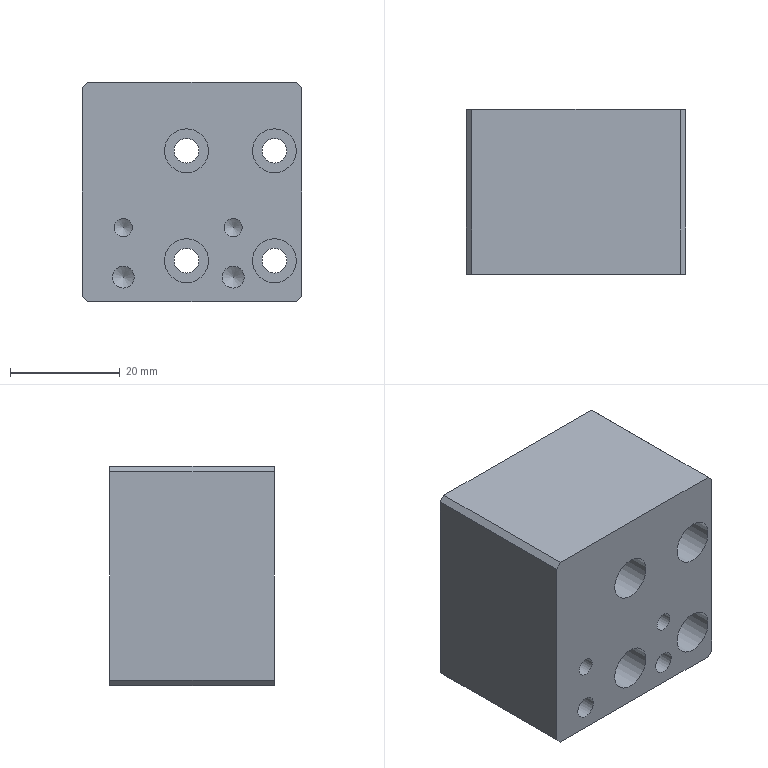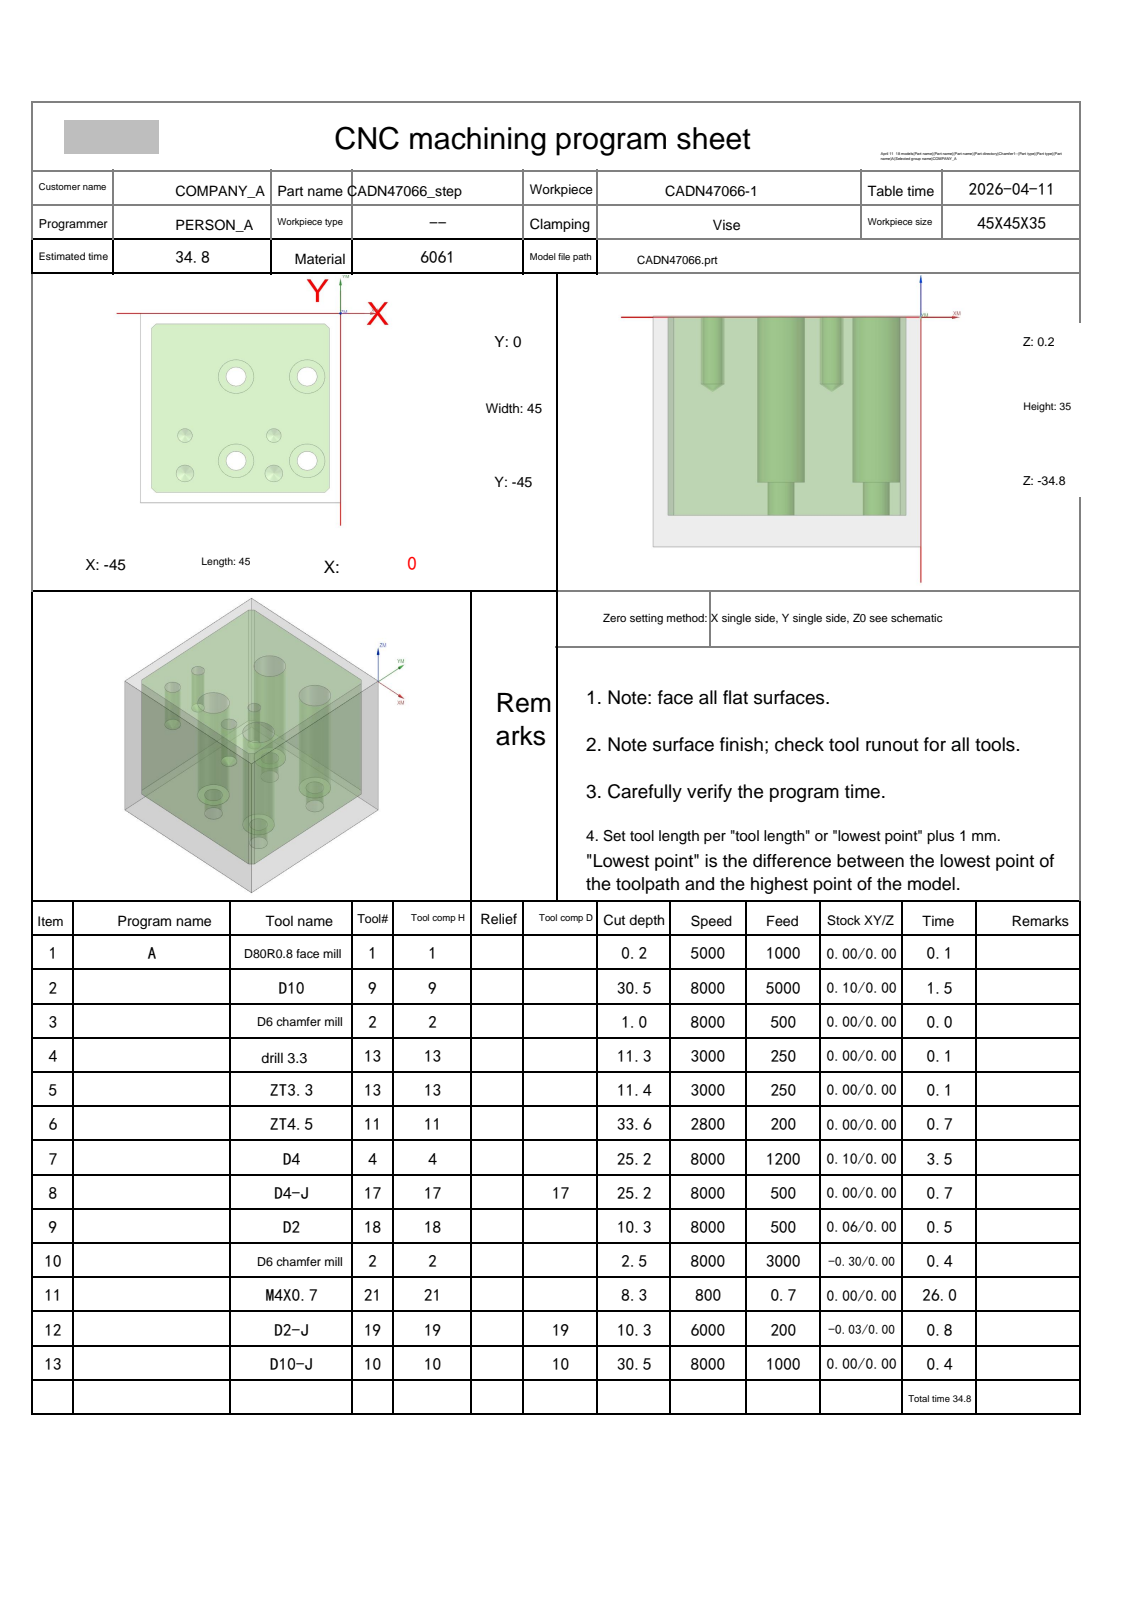NC program | NX | posted by the shop | part box 40 x 30 x 40 mm
Whole program, first 1145 of 1681 lines:
%
O0001
(Machine time: 60.64 MIN)
(===Total Tool:11===)
(T1=D80R0.8 face mill D=80.  R=0.8  D-  H01 Z=0.    )
(T9=D10     D=10.  R=0.   D-  H09 Z=-30.3 )
(T2=D6 chamfer mill   D=6.   R=0.   D-  H02 Z=-2.3  )
(T13=drill 3.3  D=3.3  DR_a=118 D-  H13 Z=-11.2 )
(T11=ZT4.5  D=4.5  DR_a=118 D-  H11 Z=-33.35)
(T4=D4      D=4.   R=0.   D-  H04 Z=-25.  )
(T17=D4-J   D=4.   R=0.   D17 H17 Z=-25.  )
(T18=D2     D=2.   R=0.   D-  H18 Z=-10.1 )
(T21=M4X0.7 D=3.3  DR_a=180 D-  H21 Z=-8.1  )
(T19=D2-J   D=2.   R=0.   D19 H19 Z=-10.1 )
(T10=D10-J  D=10.  R=0.   D10 H10 Z=-30.3 )
G80 G90 G17 G49 G40
G91 G28 Z0
M01
N1 T01 M06
(D80R0.8 face mill  D=80. R=0.8 H=01 ce=0.00 di=0.00)
G00 G90 G54 X42.5 Y-22.5 M03 S5000
G43 H01 Z20.
M08
Z2.
G01 Z0.0 F1000.
X37.5
X-82.5
X-87.5
Z2.
G00 Z20.
G91 G28 Z0.0
M05
M09
G91 G28 Z0.0
M01
N2 T09 M06
(D10  D=10. R=0. H=09 ce=0.10 di=0.00)
G00 G90 G54 X2.6 Y-22.5 M03 S8000
G43 H09 Z20.
M08
Z.5
G01 Y-41.5 Z.421 F5000.
G02 X1.106 Y-45.106 Z.404 I-5.1 J0.0
G01 X.106 Y-46.106 Z.398
G02 X-3.5 Y-47.6 Z.382 I-3.606 J3.606
G01 X-41.5 Z.223
G02 X-45.106 Y-46.106 Z.207 I0.0 J5.1
G01 X-46.106 Y-45.106 Z.201
G02 X-47.6 Y-41.5 Z.184 I3.606 J3.606
G01 Y-3.5 Z.026
G02 X-46.106 Y.106 Z.009 I5.1 J0.0
G01 X-45.106 Y1.106 Z.003
G02 X-41.5 Y2.6 Z-.013 I3.606 J-3.606
G01 X-3.5 Z-.171
G02 X.106 Y1.106 Z-.188 I0.0 J-5.1
G01 X1.106 Y.106 Z-.194
G02 X2.6 Y-3.5 Z-.211 I-3.606 J-3.606
G01 Y-41.5 Z-.369
G02 X1.106 Y-45.106 Z-.386 I-5.1 J0.0
G01 X.106 Y-46.106 Z-.391
G02 X-3.5 Y-47.6 Z-.408 I-3.606 J3.606
G01 X-41.5 Z-.566
G02 X-45.106 Y-46.106 Z-.583 I0.0 J5.1
G01 X-46.106 Y-45.106 Z-.589
G02 X-47.6 Y-41.5 Z-.606 I3.606 J3.606
G01 Y-3.5 Z-.764
G02 X-46.106 Y.106 Z-.78 I5.1 J0.0
G01 X-45.106 Y1.106 Z-.786
G02 X-41.5 Y2.6 Z-.803 I3.606 J-3.606
G01 X-3.5 Z-.961
G02 X.106 Y1.106 Z-.978 I0.0 J-5.1
G01 X1.106 Y.106 Z-.984
G02 X2.6 Y-3.5 Z-1. I-3.606 J-3.606
G01 Y-41.5 Z-1.159
G02 X1.106 Y-45.106 Z-1.175 I-5.1 J0.0
G01 X.106 Y-46.106 Z-1.181
G02 X-3.5 Y-47.6 Z-1.198 I-3.606 J3.606
G01 X-41.5 Z-1.356
G02 X-45.106 Y-46.106 Z-1.373 I0.0 J5.1
G01 X-46.106 Y-45.106 Z-1.379
G02 X-47.6 Y-41.5 Z-1.395 I3.606 J3.606
G01 Y-3.5 Z-1.553
G02 X-46.106 Y.106 Z-1.57 I5.1 J0.0
G01 X-45.106 Y1.106 Z-1.576
G02 X-41.5 Y2.6 Z-1.593 I3.606 J-3.606
G01 X-3.5 Z-1.751
G02 X.106 Y1.106 Z-1.768 I0.0 J-5.1
G01 X1.106 Y.106 Z-1.773
G02 X2.6 Y-3.5 Z-1.79 I-3.606 J-3.606
G01 Y-41.5 Z-1.948
G02 X1.106 Y-45.106 Z-1.965 I-5.1 J0.0
G01 X.106 Y-46.106 Z-1.971
G02 X-3.5 Y-47.6 Z-1.988 I-3.606 J3.606
G01 X-41.5 Z-2.146
G02 X-45.106 Y-46.106 Z-2.162 I0.0 J5.1
G01 X-46.106 Y-45.106 Z-2.168
G02 X-47.6 Y-41.5 Z-2.185 I3.606 J3.606
G01 Y-3.5 Z-2.343
G02 X-46.106 Y.106 Z-2.36 I5.1 J0.0
G01 X-45.106 Y1.106 Z-2.366
G02 X-41.5 Y2.6 Z-2.382 I3.606 J-3.606
G01 X-3.5 Z-2.541
G02 X.106 Y1.106 Z-2.557 I0.0 J-5.1
G01 X1.106 Y.106 Z-2.563
G02 X2.6 Y-3.5 Z-2.58 I-3.606 J-3.606
G01 Y-41.5 Z-2.738
G02 X1.106 Y-45.106 Z-2.755 I-5.1 J0.0
G01 X.106 Y-46.106 Z-2.761
G02 X-3.5 Y-47.6 Z-2.777 I-3.606 J3.606
G01 X-41.5 Z-2.936
G02 X-45.106 Y-46.106 Z-2.952 I0.0 J5.1
G01 X-46.106 Y-45.106 Z-2.958
G02 X-47.6 Y-41.5 Z-2.975 I3.606 J3.606
G01 Y-3.5 Z-3.133
G02 X-46.106 Y.106 Z-3.15 I5.1 J0.0
G01 X-45.106 Y1.106 Z-3.156
G02 X-41.5 Y2.6 Z-3.172 I3.606 J-3.606
G01 X-3.5 Z-3.33
G02 X.106 Y1.106 Z-3.347 I0.0 J-5.1
G01 X1.106 Y.106 Z-3.353
G02 X2.6 Y-3.5 Z-3.37 I-3.606 J-3.606
G01 Y-41.5 Z-3.528
G02 X1.106 Y-45.106 Z-3.544 I-5.1 J0.0
G01 X.106 Y-46.106 Z-3.55
G02 X-3.5 Y-47.6 Z-3.567 I-3.606 J3.606
G01 X-41.5 Z-3.725
G02 X-45.106 Y-46.106 Z-3.742 I0.0 J5.1
G01 X-46.106 Y-45.106 Z-3.748
G02 X-47.6 Y-41.5 Z-3.764 I3.606 J3.606
G01 Y-3.5 Z-3.923
G02 X-46.106 Y.106 Z-3.939 I5.1 J0.0
G01 X-45.106 Y1.106 Z-3.945
G02 X-41.5 Y2.6 Z-3.962 I3.606 J-3.606
G01 X-3.5 Z-4.12
G02 X.106 Y1.106 Z-4.137 I0.0 J-5.1
G01 X1.106 Y.106 Z-4.143
G02 X2.6 Y-3.5 Z-4.159 I-3.606 J-3.606
G01 Y-41.5 Z-4.318
G02 X1.106 Y-45.106 Z-4.334 I-5.1 J0.0
G01 X.106 Y-46.106 Z-4.34
G02 X-3.5 Y-47.6 Z-4.357 I-3.606 J3.606
G01 X-41.5 Z-4.515
G02 X-45.106 Y-46.106 Z-4.532 I0.0 J5.1
G01 X-46.106 Y-45.106 Z-4.538
G02 X-47.6 Y-41.5 Z-4.554 I3.606 J3.606
G01 Y-3.5 Z-4.712
G02 X-46.106 Y.106 Z-4.729 I5.1 J0.0
G01 X-45.106 Y1.106 Z-4.735
G02 X-41.5 Y2.6 Z-4.752 I3.606 J-3.606
G01 X-3.5 Z-4.91
G02 X.106 Y1.106 Z-4.927 I0.0 J-5.1
G01 X1.106 Y.106 Z-4.932
G02 X2.6 Y-3.5 Z-4.949 I-3.606 J-3.606
G01 Y-41.5 Z-5.107
G02 X1.106 Y-45.106 Z-5.124 I-5.1 J0.0
G01 X.106 Y-46.106 Z-5.13
G02 X-3.5 Y-47.6 Z-5.147 I-3.606 J3.606
G01 X-41.5 Z-5.305
G02 X-45.106 Y-46.106 Z-5.321 I0.0 J5.1
G01 X-46.106 Y-45.106 Z-5.327
G02 X-47.6 Y-41.5 Z-5.344 I3.606 J3.606
G01 Y-3.5 Z-5.502
G02 X-46.106 Y.106 Z-5.519 I5.1 J0.0
G01 X-45.106 Y1.106 Z-5.525
G02 X-41.5 Y2.6 Z-5.541 I3.606 J-3.606
G01 X-3.5 Z-5.7
G02 X.106 Y1.106 Z-5.716 I0.0 J-5.1
G01 X1.106 Y.106 Z-5.722
G02 X2.6 Y-3.5 Z-5.739 I-3.606 J-3.606
G01 Y-41.5 Z-5.897
G02 X1.106 Y-45.106 Z-5.914 I-5.1 J0.0
G01 X.106 Y-46.106 Z-5.92
G02 X-3.5 Y-47.6 Z-5.936 I-3.606 J3.606
G01 X-41.5 Z-6.094
G02 X-45.106 Y-46.106 Z-6.111 I0.0 J5.1
G01 X-46.106 Y-45.106 Z-6.117
G02 X-47.6 Y-41.5 Z-6.134 I3.606 J3.606
G01 Y-3.5 Z-6.292
G02 X-46.106 Y.106 Z-6.309 I5.1 J0.0
G01 X-45.106 Y1.106 Z-6.314
G02 X-41.5 Y2.6 Z-6.331 I3.606 J-3.606
G01 X-3.5 Z-6.489
G02 X.106 Y1.106 Z-6.506 I0.0 J-5.1
G01 X1.106 Y.106 Z-6.512
G02 X2.6 Y-3.5 Z-6.529 I-3.606 J-3.606
G01 Y-41.5 Z-6.687
G02 X1.106 Y-45.106 Z-6.703 I-5.1 J0.0
G01 X.106 Y-46.106 Z-6.709
G02 X-3.5 Y-47.6 Z-6.726 I-3.606 J3.606
G01 X-41.5 Z-6.884
G02 X-45.106 Y-46.106 Z-6.901 I0.0 J5.1
G01 X-46.106 Y-45.106 Z-6.907
G02 X-47.6 Y-41.5 Z-6.923 I3.606 J3.606
G01 Y-3.5 Z-7.082
G02 X-46.106 Y.106 Z-7.098 I5.1 J0.0
G01 X-45.106 Y1.106 Z-7.104
G02 X-41.5 Y2.6 Z-7.121 I3.606 J-3.606
G01 X-3.5 Z-7.279
G02 X.106 Y1.106 Z-7.296 I0.0 J-5.1
G01 X1.106 Y.106 Z-7.302
G02 X2.6 Y-3.5 Z-7.318 I-3.606 J-3.606
G01 Y-41.5 Z-7.477
G02 X1.106 Y-45.106 Z-7.493 I-5.1 J0.0
G01 X.106 Y-46.106 Z-7.499
G02 X-3.5 Y-47.6 Z-7.516 I-3.606 J3.606
G01 X-41.5 Z-7.674
G02 X-45.106 Y-46.106 Z-7.691 I0.0 J5.1
G01 X-46.106 Y-45.106 Z-7.697
G02 X-47.6 Y-41.5 Z-7.713 I3.606 J3.606
G01 Y-3.5 Z-7.871
G02 X-46.106 Y.106 Z-7.888 I5.1 J0.0
G01 X-45.106 Y1.106 Z-7.894
G02 X-41.5 Y2.6 Z-7.911 I3.606 J-3.606
G01 X-3.5 Z-8.069
G02 X.106 Y1.106 Z-8.086 I0.0 J-5.1
G01 X1.106 Y.106 Z-8.091
G02 X2.6 Y-3.5 Z-8.108 I-3.606 J-3.606
G01 Y-41.5 Z-8.266
G02 X1.106 Y-45.106 Z-8.283 I-5.1 J0.0
G01 X.106 Y-46.106 Z-8.289
G02 X-3.5 Y-47.6 Z-8.306 I-3.606 J3.606
G01 X-41.5 Z-8.464
G02 X-45.106 Y-46.106 Z-8.48 I0.0 J5.1
G01 X-46.106 Y-45.106 Z-8.486
G02 X-47.6 Y-41.5 Z-8.503 I3.606 J3.606
G01 Y-3.5 Z-8.661
G02 X-46.106 Y.106 Z-8.678 I5.1 J0.0
G01 X-45.106 Y1.106 Z-8.684
G02 X-41.5 Y2.6 Z-8.7 I3.606 J-3.606
G01 X-3.5 Z-8.859
G02 X.106 Y1.106 Z-8.875 I0.0 J-5.1
G01 X1.106 Y.106 Z-8.881
G02 X2.6 Y-3.5 Z-8.898 I-3.606 J-3.606
G01 Y-41.5 Z-9.056
G02 X1.106 Y-45.106 Z-9.073 I-5.1 J0.0
G01 X.106 Y-46.106 Z-9.079
G02 X-3.5 Y-47.6 Z-9.095 I-3.606 J3.606
G01 X-41.5 Z-9.253
G02 X-45.106 Y-46.106 Z-9.27 I0.0 J5.1
G01 X-46.106 Y-45.106 Z-9.276
G02 X-47.6 Y-41.5 Z-9.293 I3.606 J3.606
G01 Y-3.5 Z-9.451
G02 X-46.106 Y.106 Z-9.468 I5.1 J0.0
G01 X-45.106 Y1.106 Z-9.473
G02 X-41.5 Y2.6 Z-9.49 I3.606 J-3.606
G01 X-3.5 Z-9.648
G02 X.106 Y1.106 Z-9.665 I0.0 J-5.1
G01 X1.106 Y.106 Z-9.671
G02 X2.6 Y-3.5 Z-9.688 I-3.606 J-3.606
G01 Y-41.5 Z-9.846
G02 X1.106 Y-45.106 Z-9.862 I-5.1 J0.0
G01 X.106 Y-46.106 Z-9.868
G02 X-3.5 Y-47.6 Z-9.885 I-3.606 J3.606
G01 X-41.5 Z-10.043
G02 X-45.106 Y-46.106 Z-10.06 I0.0 J5.1
G01 X-46.106 Y-45.106 Z-10.066
G02 X-47.6 Y-41.5 Z-10.082 I3.606 J3.606
G01 Y-3.5 Z-10.241
G02 X-46.106 Y.106 Z-10.257 I5.1 J0.0
G01 X-45.106 Y1.106 Z-10.263
G02 X-41.5 Y2.6 Z-10.28 I3.606 J-3.606
G01 X-3.5 Z-10.438
G02 X.106 Y1.106 Z-10.455 I0.0 J-5.1
G01 X1.106 Y.106 Z-10.461
G02 X2.6 Y-3.5 Z-10.477 I-3.606 J-3.606
G01 Y-41.5 Z-10.636
G02 X1.106 Y-45.106 Z-10.652 I-5.1 J0.0
G01 X.106 Y-46.106 Z-10.658
G02 X-3.5 Y-47.6 Z-10.675 I-3.606 J3.606
G01 X-41.5 Z-10.833
G02 X-45.106 Y-46.106 Z-10.85 I0.0 J5.1
G01 X-46.106 Y-45.106 Z-10.856
G02 X-47.6 Y-41.5 Z-10.872 I3.606 J3.606
G01 Y-3.5 Z-11.03
G02 X-46.106 Y.106 Z-11.047 I5.1 J0.0
G01 X-45.106 Y1.106 Z-11.053
G02 X-41.5 Y2.6 Z-11.07 I3.606 J-3.606
G01 X-3.5 Z-11.228
G02 X.106 Y1.106 Z-11.244 I0.0 J-5.1
G01 X1.106 Y.106 Z-11.25
G02 X2.6 Y-3.5 Z-11.267 I-3.606 J-3.606
G01 Y-41.5 Z-11.425
G02 X1.106 Y-45.106 Z-11.442 I-5.1 J0.0
G01 X.106 Y-46.106 Z-11.448
G02 X-3.5 Y-47.6 Z-11.464 I-3.606 J3.606
G01 X-41.5 Z-11.623
G02 X-45.106 Y-46.106 Z-11.639 I0.0 J5.1
G01 X-46.106 Y-45.106 Z-11.645
G02 X-47.6 Y-41.5 Z-11.662 I3.606 J3.606
G01 Y-3.5 Z-11.82
G02 X-46.106 Y.106 Z-11.837 I5.1 J0.0
G01 X-45.106 Y1.106 Z-11.843
G02 X-41.5 Y2.6 Z-11.859 I3.606 J-3.606
G01 X-3.5 Z-12.018
G02 X.106 Y1.106 Z-12.034 I0.0 J-5.1
G01 X1.106 Y.106 Z-12.04
G02 X2.6 Y-3.5 Z-12.057 I-3.606 J-3.606
G01 Y-41.5 Z-12.215
G02 X1.106 Y-45.106 Z-12.232 I-5.1 J0.0
G01 X.106 Y-46.106 Z-12.238
G02 X-3.5 Y-47.6 Z-12.254 I-3.606 J3.606
G01 X-41.5 Z-12.412
G02 X-45.106 Y-46.106 Z-12.429 I0.0 J5.1
G01 X-46.106 Y-45.106 Z-12.435
G02 X-47.6 Y-41.5 Z-12.452 I3.606 J3.606
G01 Y-3.5 Z-12.61
G02 X-46.106 Y.106 Z-12.627 I5.1 J0.0
G01 X-45.106 Y1.106 Z-12.632
G02 X-41.5 Y2.6 Z-12.649 I3.606 J-3.606
G01 X-3.5 Z-12.807
G02 X.106 Y1.106 Z-12.824 I0.0 J-5.1
G01 X1.106 Y.106 Z-12.83
G02 X2.6 Y-3.5 Z-12.847 I-3.606 J-3.606
G01 Y-41.5 Z-13.005
G02 X1.106 Y-45.106 Z-13.021 I-5.1 J0.0
G01 X.106 Y-46.106 Z-13.027
G02 X-3.5 Y-47.6 Z-13.044 I-3.606 J3.606
G01 X-41.5 Z-13.202
G02 X-45.106 Y-46.106 Z-13.219 I0.0 J5.1
G01 X-46.106 Y-45.106 Z-13.225
G02 X-47.6 Y-41.5 Z-13.241 I3.606 J3.606
G01 Y-3.5 Z-13.4
G02 X-46.106 Y.106 Z-13.416 I5.1 J0.0
G01 X-45.106 Y1.106 Z-13.422
G02 X-41.5 Y2.6 Z-13.439 I3.606 J-3.606
G01 X-3.5 Z-13.597
G02 X.106 Y1.106 Z-13.614 I0.0 J-5.1
G01 X1.106 Y.106 Z-13.62
G02 X2.6 Y-3.5 Z-13.636 I-3.606 J-3.606
G01 Y-41.5 Z-13.794
G02 X1.106 Y-45.106 Z-13.811 I-5.1 J0.0
G01 X.106 Y-46.106 Z-13.817
G02 X-3.5 Y-47.6 Z-13.834 I-3.606 J3.606
G01 X-41.5 Z-13.992
G02 X-45.106 Y-46.106 Z-14.009 I0.0 J5.1
G01 X-46.106 Y-45.106 Z-14.014
G02 X-47.6 Y-41.5 Z-14.031 I3.606 J3.606
G01 Y-3.5 Z-14.189
G02 X-46.106 Y.106 Z-14.206 I5.1 J0.0
G01 X-45.106 Y1.106 Z-14.212
G02 X-41.5 Y2.6 Z-14.229 I3.606 J-3.606
G01 X-3.5 Z-14.387
G02 X.106 Y1.106 Z-14.403 I0.0 J-5.1
G01 X1.106 Y.106 Z-14.409
G02 X2.6 Y-3.5 Z-14.426 I-3.606 J-3.606
G01 Y-41.5 Z-14.584
G02 X1.106 Y-45.106 Z-14.601 I-5.1 J0.0
G01 X.106 Y-46.106 Z-14.607
G02 X-3.5 Y-47.6 Z-14.623 I-3.606 J3.606
G01 X-41.5 Z-14.782
G02 X-45.106 Y-46.106 Z-14.798 I0.0 J5.1
G01 X-46.106 Y-45.106 Z-14.804
G02 X-47.6 Y-41.5 Z-14.821 I3.606 J3.606
G01 Y-3.5 Z-14.979
G02 X-46.106 Y.106 Z-14.996 I5.1 J0.0
G01 X-45.106 Y1.106 Z-15.002
G02 X-41.5 Y2.6 Z-15.018 I3.606 J-3.606
G01 X-3.5 Z-15.177
G02 X.106 Y1.106 Z-15.193 I0.0 J-5.1
G01 X1.106 Y.106 Z-15.199
G02 X2.6 Y-3.5 Z-15.216 I-3.606 J-3.606
G01 Y-41.5 Z-15.374
G02 X1.106 Y-45.106 Z-15.391 I-5.1 J0.0
G01 X.106 Y-46.106 Z-15.397
G02 X-3.5 Y-47.6 Z-15.413 I-3.606 J3.606
G01 X-41.5 Z-15.571
G02 X-45.106 Y-46.106 Z-15.588 I0.0 J5.1
G01 X-46.106 Y-45.106 Z-15.594
G02 X-47.6 Y-41.5 Z-15.611 I3.606 J3.606
G01 Y-3.5 Z-15.769
G02 X-46.106 Y.106 Z-15.786 I5.1 J0.0
G01 X-45.106 Y1.106 Z-15.791
G02 X-41.5 Y2.6 Z-15.808 I3.606 J-3.606
G01 X-3.5 Z-15.966
G02 X.106 Y1.106 Z-15.983 I0.0 J-5.1
G01 X1.106 Y.106 Z-15.989
G02 X2.6 Y-3.5 Z-16.006 I-3.606 J-3.606
G01 Y-41.5 Z-16.164
G02 X1.106 Y-45.106 Z-16.18 I-5.1 J0.0
G01 X.106 Y-46.106 Z-16.186
G02 X-3.5 Y-47.6 Z-16.203 I-3.606 J3.606
G01 X-41.5 Z-16.361
G02 X-45.106 Y-46.106 Z-16.378 I0.0 J5.1
G01 X-46.106 Y-45.106 Z-16.384
G02 X-47.6 Y-41.5 Z-16.4 I3.606 J3.606
G01 Y-3.5 Z-16.559
G02 X-46.106 Y.106 Z-16.575 I5.1 J0.0
G01 X-45.106 Y1.106 Z-16.581
G02 X-41.5 Y2.6 Z-16.598 I3.606 J-3.606
G01 X-3.5 Z-16.756
G02 X.106 Y1.106 Z-16.773 I0.0 J-5.1
G01 X1.106 Y.106 Z-16.779
G02 X2.6 Y-3.5 Z-16.795 I-3.606 J-3.606
G01 Y-41.5 Z-16.953
G02 X1.106 Y-45.106 Z-16.97 I-5.1 J0.0
G01 X.106 Y-46.106 Z-16.976
G02 X-3.5 Y-47.6 Z-16.993 I-3.606 J3.606
G01 X-41.5 Z-17.151
G02 X-45.106 Y-46.106 Z-17.168 I0.0 J5.1
G01 X-46.106 Y-45.106 Z-17.173
G02 X-47.6 Y-41.5 Z-17.19 I3.606 J3.606
G01 Y-3.5 Z-17.348
G02 X-46.106 Y.106 Z-17.365 I5.1 J0.0
G01 X-45.106 Y1.106 Z-17.371
G02 X-41.5 Y2.6 Z-17.388 I3.606 J-3.606
G01 X-3.5 Z-17.546
G02 X.106 Y1.106 Z-17.562 I0.0 J-5.1
G01 X1.106 Y.106 Z-17.568
G02 X2.6 Y-3.5 Z-17.585 I-3.606 J-3.606
G01 Y-41.5 Z-17.743
G02 X1.106 Y-45.106 Z-17.76 I-5.1 J0.0
G01 X.106 Y-46.106 Z-17.766
G02 X-3.5 Y-47.6 Z-17.782 I-3.606 J3.606
G01 X-41.5 Z-17.941
G02 X-45.106 Y-46.106 Z-17.957 I0.0 J5.1
G01 X-46.106 Y-45.106 Z-17.963
G02 X-47.6 Y-41.5 Z-17.98 I3.606 J3.606
G01 Y-3.5 Z-18.138
G02 X-46.106 Y.106 Z-18.155 I5.1 J0.0
G01 X-45.106 Y1.106 Z-18.161
G02 X-41.5 Y2.6 Z-18.177 I3.606 J-3.606
G01 X-3.5 Z-18.336
G02 X.106 Y1.106 Z-18.352 I0.0 J-5.1
G01 X1.106 Y.106 Z-18.358
G02 X2.6 Y-3.5 Z-18.375 I-3.606 J-3.606
G01 Y-41.5 Z-18.533
G02 X1.106 Y-45.106 Z-18.55 I-5.1 J0.0
G01 X.106 Y-46.106 Z-18.556
G02 X-3.5 Y-47.6 Z-18.572 I-3.606 J3.606
G01 X-41.5 Z-18.73
G02 X-45.106 Y-46.106 Z-18.747 I0.0 J5.1
G01 X-46.106 Y-45.106 Z-18.753
G02 X-47.6 Y-41.5 Z-18.77 I3.606 J3.606
G01 Y-3.5 Z-18.928
G02 X-46.106 Y.106 Z-18.944 I5.1 J0.0
G01 X-45.106 Y1.106 Z-18.95
G02 X-41.5 Y2.6 Z-18.967 I3.606 J-3.606
G01 X-3.5 Z-19.125
G02 X.106 Y1.106 Z-19.142 I0.0 J-5.1
G01 X1.106 Y.106 Z-19.148
G02 X2.6 Y-3.5 Z-19.164 I-3.606 J-3.606
G01 Y-41.5 Z-19.323
G02 X1.106 Y-45.106 Z-19.339 I-5.1 J0.0
G01 X.106 Y-46.106 Z-19.345
G02 X-3.5 Y-47.6 Z-19.362 I-3.606 J3.606
G01 X-41.5 Z-19.52
G02 X-45.106 Y-46.106 Z-19.537 I0.0 J5.1
G01 X-46.106 Y-45.106 Z-19.543
G02 X-47.6 Y-41.5 Z-19.559 I3.606 J3.606
G01 Y-3.5 Z-19.718
G02 X-46.106 Y.106 Z-19.734 I5.1 J0.0
G01 X-45.106 Y1.106 Z-19.74
G02 X-41.5 Y2.6 Z-19.757 I3.606 J-3.606
G01 X-3.5 Z-19.915
G02 X.106 Y1.106 Z-19.932 I0.0 J-5.1
G01 X1.106 Y.106 Z-19.938
G02 X2.6 Y-3.5 Z-19.954 I-3.606 J-3.606
G01 Y-41.5 Z-20.112
G02 X1.106 Y-45.106 Z-20.129 I-5.1 J0.0
G01 X.106 Y-46.106 Z-20.135
G02 X-3.5 Y-47.6 Z-20.152 I-3.606 J3.606
G01 X-41.5 Z-20.31
G02 X-45.106 Y-46.106 Z-20.327 I0.0 J5.1
G01 X-46.106 Y-45.106 Z-20.332
G02 X-47.6 Y-41.5 Z-20.349 I3.606 J3.606
G01 Y-3.5 Z-20.507
G02 X-46.106 Y.106 Z-20.524 I5.1 J0.0
G01 X-45.106 Y1.106 Z-20.53
G02 X-41.5 Y2.6 Z-20.547 I3.606 J-3.606
G01 X-3.5 Z-20.705
G02 X.106 Y1.106 Z-20.721 I0.0 J-5.1
G01 X1.106 Y.106 Z-20.727
G02 X2.6 Y-3.5 Z-20.744 I-3.606 J-3.606
G01 Y-41.5 Z-20.902
G02 X1.106 Y-45.106 Z-20.919 I-5.1 J0.0
G01 X.106 Y-46.106 Z-20.925
G02 X-3.5 Y-47.6 Z-20.941 I-3.606 J3.606
G01 X-41.5 Z-21.1
G02 X-45.106 Y-46.106 Z-21.116 I0.0 J5.1
G01 X-46.106 Y-45.106 Z-21.122
G02 X-47.6 Y-41.5 Z-21.139 I3.606 J3.606
G01 Y-3.5 Z-21.297
G02 X-46.106 Y.106 Z-21.314 I5.1 J0.0
G01 X-45.106 Y1.106 Z-21.32
G02 X-41.5 Y2.6 Z-21.336 I3.606 J-3.606
G01 X-3.5 Z-21.494
G02 X.106 Y1.106 Z-21.511 I0.0 J-5.1
G01 X1.106 Y.106 Z-21.517
G02 X2.6 Y-3.5 Z-21.534 I-3.606 J-3.606
G01 Y-41.5 Z-21.692
G02 X1.106 Y-45.106 Z-21.709 I-5.1 J0.0
G01 X.106 Y-46.106 Z-21.714
G02 X-3.5 Y-47.6 Z-21.731 I-3.606 J3.606
G01 X-41.5 Z-21.889
G02 X-45.106 Y-46.106 Z-21.906 I0.0 J5.1
G01 X-46.106 Y-45.106 Z-21.912
G02 X-47.6 Y-41.5 Z-21.929 I3.606 J3.606
G01 Y-3.5 Z-22.087
G02 X-46.106 Y.106 Z-22.103 I5.1 J0.0
G01 X-45.106 Y1.106 Z-22.109
G02 X-41.5 Y2.6 Z-22.126 I3.606 J-3.606
G01 X-3.5 Z-22.284
G02 X.106 Y1.106 Z-22.301 I0.0 J-5.1
G01 X1.106 Y.106 Z-22.307
G02 X2.6 Y-3.5 Z-22.323 I-3.606 J-3.606
G01 Y-41.5 Z-22.482
G02 X1.106 Y-45.106 Z-22.498 I-5.1 J0.0
G01 X.106 Y-46.106 Z-22.504
G02 X-3.5 Y-47.6 Z-22.521 I-3.606 J3.606
G01 X-41.5 Z-22.679
G02 X-45.106 Y-46.106 Z-22.696 I0.0 J5.1
G01 X-46.106 Y-45.106 Z-22.702
G02 X-47.6 Y-41.5 Z-22.718 I3.606 J3.606
G01 Y-3.5 Z-22.877
G02 X-46.106 Y.106 Z-22.893 I5.1 J0.0
G01 X-45.106 Y1.106 Z-22.899
G02 X-41.5 Y2.6 Z-22.916 I3.606 J-3.606
G01 X-3.5 Z-23.074
G02 X.106 Y1.106 Z-23.091 I0.0 J-5.1
G01 X1.106 Y.106 Z-23.097
G02 X2.6 Y-3.5 Z-23.113 I-3.606 J-3.606
G01 Y-41.5 Z-23.271
G02 X1.106 Y-45.106 Z-23.288 I-5.1 J0.0
G01 X.106 Y-46.106 Z-23.294
G02 X-3.5 Y-47.6 Z-23.311 I-3.606 J3.606
G01 X-41.5 Z-23.469
G02 X-45.106 Y-46.106 Z-23.486 I0.0 J5.1
G01 X-46.106 Y-45.106 Z-23.491
G02 X-47.6 Y-41.5 Z-23.508 I3.606 J3.606
G01 Y-3.5 Z-23.666
G02 X-46.106 Y.106 Z-23.683 I5.1 J0.0
G01 X-45.106 Y1.106 Z-23.689
G02 X-41.5 Y2.6 Z-23.706 I3.606 J-3.606
G01 X-3.5 Z-23.864
G02 X.106 Y1.106 Z-23.88 I0.0 J-5.1
G01 X1.106 Y.106 Z-23.886
G02 X2.6 Y-3.5 Z-23.903 I-3.606 J-3.606
G01 Y-41.5 Z-24.061
G02 X1.106 Y-45.106 Z-24.078 I-5.1 J0.0
G01 X.106 Y-46.106 Z-24.084
G02 X-3.5 Y-47.6 Z-24.1 I-3.606 J3.606
G01 X-41.5 Z-24.259
G02 X-45.106 Y-46.106 Z-24.275 I0.0 J5.1
G01 X-46.106 Y-45.106 Z-24.281
G02 X-47.6 Y-41.5 Z-24.298 I3.606 J3.606
G01 Y-3.5 Z-24.456
G02 X-46.106 Y.106 Z-24.473 I5.1 J0.0
G01 X-45.106 Y1.106 Z-24.479
G02 X-41.5 Y2.6 Z-24.495 I3.606 J-3.606
G01 X-3.5 Z-24.653
G02 X.106 Y1.106 Z-24.67 I0.0 J-5.1
G01 X1.106 Y.106 Z-24.676
G02 X2.6 Y-3.5 Z-24.693 I-3.606 J-3.606
G01 Y-41.5 Z-24.851
G02 X1.106 Y-45.106 Z-24.868 I-5.1 J0.0
G01 X.106 Y-46.106 Z-24.873
G02 X-3.5 Y-47.6 Z-24.89 I-3.606 J3.606
G01 X-41.5 Z-25.048
G02 X-45.106 Y-46.106 Z-25.065 I0.0 J5.1
G01 X-46.106 Y-45.106 Z-25.071
G02 X-47.6 Y-41.5 Z-25.088 I3.606 J3.606
G01 Y-3.5 Z-25.246
G02 X-46.106 Y.106 Z-25.262 I5.1 J0.0
G01 X-45.106 Y1.106 Z-25.268
G02 X-41.5 Y2.6 Z-25.285 I3.606 J-3.606
G01 X-3.5 Z-25.443
G02 X.106 Y1.106 Z-25.46 I0.0 J-5.1
G01 X1.106 Y.106 Z-25.466
G02 X2.6 Y-3.5 Z-25.482 I-3.606 J-3.606
G01 Y-41.5 Z-25.641
G02 X1.106 Y-45.106 Z-25.657 I-5.1 J0.0
G01 X.106 Y-46.106 Z-25.663
G02 X-3.5 Y-47.6 Z-25.68 I-3.606 J3.606
G01 X-41.5 Z-25.838
G02 X-45.106 Y-46.106 Z-25.855 I0.0 J5.1
G01 X-46.106 Y-45.106 Z-25.861
G02 X-47.6 Y-41.5 Z-25.877 I3.606 J3.606
G01 Y-3.5 Z-26.036
G02 X-46.106 Y.106 Z-26.052 I5.1 J0.0
G01 X-45.106 Y1.106 Z-26.058
G02 X-41.5 Y2.6 Z-26.075 I3.606 J-3.606
G01 X-3.5 Z-26.233
G02 X.106 Y1.106 Z-26.25 I0.0 J-5.1
G01 X1.106 Y.106 Z-26.256
G02 X2.6 Y-3.5 Z-26.272 I-3.606 J-3.606
G01 Y-41.5 Z-26.43
G02 X1.106 Y-45.106 Z-26.447 I-5.1 J0.0
G01 X.106 Y-46.106 Z-26.453
G02 X-3.5 Y-47.6 Z-26.47 I-3.606 J3.606
G01 X-41.5 Z-26.628
G02 X-45.106 Y-46.106 Z-26.644 I0.0 J5.1
G01 X-46.106 Y-45.106 Z-26.65
G02 X-47.6 Y-41.5 Z-26.667 I3.606 J3.606
G01 Y-3.5 Z-26.825
G02 X-46.106 Y.106 Z-26.842 I5.1 J0.0
G01 X-45.106 Y1.106 Z-26.848
G02 X-41.5 Y2.6 Z-26.864 I3.606 J-3.606
G01 X-3.5 Z-27.023
G02 X.106 Y1.106 Z-27.039 I0.0 J-5.1
G01 X1.106 Y.106 Z-27.045
G02 X2.6 Y-3.5 Z-27.062 I-3.606 J-3.606
G01 Y-41.5 Z-27.22
G02 X1.106 Y-45.106 Z-27.237 I-5.1 J0.0
G01 X.106 Y-46.106 Z-27.243
G02 X-3.5 Y-47.6 Z-27.259 I-3.606 J3.606
G01 X-41.5 Z-27.418
G02 X-45.106 Y-46.106 Z-27.434 I0.0 J5.1
G01 X-46.106 Y-45.106 Z-27.44
G02 X-47.6 Y-41.5 Z-27.457 I3.606 J3.606
G01 Y-3.5 Z-27.615
G02 X-46.106 Y.106 Z-27.632 I5.1 J0.0
G01 X-45.106 Y1.106 Z-27.638
G02 X-41.5 Y2.6 Z-27.654 I3.606 J-3.606
G01 X-3.5 Z-27.812
G02 X.106 Y1.106 Z-27.829 I0.0 J-5.1
G01 X1.106 Y.106 Z-27.835
G02 X2.6 Y-3.5 Z-27.852 I-3.606 J-3.606
G01 Y-41.5 Z-28.01
G02 X1.106 Y-45.106 Z-28.027 I-5.1 J0.0
G01 X.106 Y-46.106 Z-28.032
G02 X-3.5 Y-47.6 Z-28.049 I-3.606 J3.606
G01 X-41.5 Z-28.207
G02 X-45.106 Y-46.106 Z-28.224 I0.0 J5.1
G01 X-46.106 Y-45.106 Z-28.23
G02 X-47.6 Y-41.5 Z-28.247 I3.606 J3.606
G01 Y-3.5 Z-28.405
G02 X-46.106 Y.106 Z-28.421 I5.1 J0.0
G01 X-45.106 Y1.106 Z-28.427
G02 X-41.5 Y2.6 Z-28.444 I3.606 J-3.606
G01 X-3.5 Z-28.602
G02 X.106 Y1.106 Z-28.619 I0.0 J-5.1
G01 X1.106 Y.106 Z-28.625
G02 X2.6 Y-3.5 Z-28.641 I-3.606 J-3.606
G01 Y-41.5 Z-28.8
G02 X1.106 Y-45.106 Z-28.816 I-5.1 J0.0
G01 X.106 Y-46.106 Z-28.822
G02 X-3.5 Y-47.6 Z-28.839 I-3.606 J3.606
G01 X-41.5 Z-28.997
G02 X-45.106 Y-46.106 Z-29.014 I0.0 J5.1
G01 X-46.106 Y-45.106 Z-29.02
G02 X-47.6 Y-41.5 Z-29.036 I3.606 J3.606
G01 Y-3.5 Z-29.194
G02 X-46.106 Y.106 Z-29.211 I5.1 J0.0
G01 X-45.106 Y1.106 Z-29.217
G02 X-41.5 Y2.6 Z-29.234 I3.606 J-3.606
G01 X-3.5 Z-29.392
G02 X.106 Y1.106 Z-29.409 I0.0 J-5.1
G01 X1.106 Y.106 Z-29.414
G02 X2.6 Y-3.5 Z-29.431 I-3.606 J-3.606
G01 Y-41.5 Z-29.589
G02 X1.106 Y-45.106 Z-29.606 I-5.1 J0.0
G01 X.106 Y-46.106 Z-29.612
G02 X-3.5 Y-47.6 Z-29.629 I-3.606 J3.606
G01 X-41.5 Z-29.787
G02 X-45.106 Y-46.106 Z-29.803 I0.0 J5.1
G01 X-46.106 Y-45.106 Z-29.809
G02 X-47.6 Y-41.5 Z-29.826 I3.606 J3.606
G01 Y-3.5 Z-29.984
G02 X-46.106 Y.106 Z-30.001 I5.1 J0.0
G01 X-45.106 Y1.106 Z-30.007
G02 X-41.5 Y2.6 Z-30.023 I3.606 J-3.606
G01 X-3.5 Z-30.182
G02 X.106 Y1.106 Z-30.198 I0.0 J-5.1
G01 X1.106 Y.106 Z-30.204
G02 X2.6 Y-3.5 Z-30.221 I-3.606 J-3.606
G01 Y-22.5 Z-30.3
Y-41.5
G02 X1.106 Y-45.106 I-5.1 J0.0
G01 X.106 Y-46.106
G02 X-3.5 Y-47.6 I-3.606 J3.606
G01 X-41.5
G02 X-45.106 Y-46.106 I0.0 J5.1
G01 X-46.106 Y-45.106
G02 X-47.6 Y-41.5 I3.606 J3.606
G01 Y-3.5
G02 X-46.106 Y.106 I5.1 J0.0
G01 X-45.106 Y1.106
G02 X-41.5 Y2.6 I3.606 J-3.606
G01 X-3.5
G02 X.106 Y1.106 I0.0 J-5.1
G01 X1.106 Y.106
G02 X2.6 Y-3.5 I-3.606 J-3.606
G01 Y-22.5
Y-23.
Z-29.3
G00 Z20.
G91 G28 Z0.0
M05
M09
G91 G28 Z0.0
M01
N3 T02 M06
(D6 chamfer mill  D=6. R=0. H=02 ce=0.00 di=0.00)
G00 G90 G54 X-35. Y-29. M03 S8000
G43 H02 Z20.
M08
G98 G81 X-35. Y-29. Z-.8 R1. F500.
Y-38.
X-23.5 Y-35.
X-15. Y-38.
X-7.5 Y-35.
X-15. Y-29.
X-7.5 Y-15.
X-23.5
G80
G00 Z20.
G91 G28 Z0.0
M05
M09
G91 G28 Z0.0
M01
N4 T13 M06
(drill 3.3 D=3.3 DR_a=118 H=13)
G00 G90 G54 X-35. Y-29. M03 S3000
G43 H13 Z20.
M08
G98 G83 X-35. Y-29. Z-11.091 R1. F250. Q2.
X-15.
G80
G00 Z20.
G91 G28 Z0.0
M05
M09
G91 G28 Z0.0
M01
N5 T13 M06
(ZT3.3 D=3.3 DR_a=118 H=13)
G00 G90 G54 X-35. Y-38. M03 S3000
G43 H13 Z20.
M08
G98 G83 X-35. Y-38. Z-11.202 R1. F250. Q2.
X-15.
G80
G00 Z20.
G91 G28 Z0.0
M05
M09
G91 G28 Z0.0
M01
N6 T11 M06
(ZT4.5 D=4.5 DR_a=118 H=11)
G00 G90 G54 X-23.5 Y-15. M03 S2800
G43 H11 Z20.
M08
G98 G83 X-23.5 Y-15. Z-33.352 R1. F200. Q2.
X-7.5
Y-35.
X-23.5
G80
G00 Z20.
G91 G28 Z0.0
M05
M09
G91 G28 Z0.0
M01
N7 T04 M06
(D4  D=4. R=0. H=04 ce=0.10 di=0.00)
G00 G90 G54 X-23.5 Y-15. M03 S8000
G43 H04 Z20.
M08
Z.5
G03 X-22.55 Y-15.95 I.95 J0.0 F1200.
X-21.6 Y-15. I0.0 J.95
X-21.6 Y-15. Z.2 I-1.9 J0.0
X-21.6 Y-15. Z-.1 I-1.9 J0.0
X-21.6 Y-15. Z-.4 I-1.9 J0.0
X-21.6 Y-15. Z-.7 I-1.9 J0.0
X-21.6 Y-15. Z-1. I-1.9 J0.0
X-21.6 Y-15. Z-1.3 I-1.9 J0.0
X-21.6 Y-15. Z-1.6 I-1.9 J0.0
X-21.6 Y-15. Z-1.9 I-1.9 J0.0
X-21.6 Y-15. Z-2.2 I-1.9 J0.0
X-21.6 Y-15. Z-2.5 I-1.9 J0.0
X-21.6 Y-15. Z-2.8 I-1.9 J0.0
X-21.6 Y-15. Z-3.1 I-1.9 J0.0
X-21.6 Y-15. Z-3.4 I-1.9 J0.0
X-21.6 Y-15. Z-3.7 I-1.9 J0.0
X-21.6 Y-15. Z-4. I-1.9 J0.0
X-21.6 Y-15. Z-4.3 I-1.9 J0.0
X-21.6 Y-15. Z-4.6 I-1.9 J0.0
X-21.6 Y-15. Z-4.9 I-1.9 J0.0
X-21.6 Y-15. Z-5.2 I-1.9 J0.0
X-21.6 Y-15. Z-5.5 I-1.9 J0.0
X-21.6 Y-15. Z-5.8 I-1.9 J0.0
X-21.6 Y-15. Z-6.1 I-1.9 J0.0
X-21.6 Y-15. Z-6.4 I-1.9 J0.0
X-21.6 Y-15. Z-6.7 I-1.9 J0.0
X-21.6 Y-15. Z-7. I-1.9 J0.0
X-21.6 Y-15. Z-7.3 I-1.9 J0.0
X-21.6 Y-15. Z-7.6 I-1.9 J0.0
X-21.6 Y-15. Z-7.9 I-1.9 J0.0
X-21.6 Y-15. Z-8.2 I-1.9 J0.0
X-21.6 Y-15. Z-8.5 I-1.9 J0.0
X-21.6 Y-15. Z-8.8 I-1.9 J0.0
X-21.6 Y-15. Z-9.1 I-1.9 J0.0
X-21.6 Y-15. Z-9.4 I-1.9 J0.0
X-21.6 Y-15. Z-9.7 I-1.9 J0.0
X-21.6 Y-15. Z-10. I-1.9 J0.0
X-21.6 Y-15. Z-10.3 I-1.9 J0.0
X-21.6 Y-15. Z-10.6 I-1.9 J0.0
X-21.6 Y-15. Z-10.9 I-1.9 J0.0
X-21.6 Y-15. Z-11.2 I-1.9 J0.0
X-21.6 Y-15. Z-11.5 I-1.9 J0.0
X-21.6 Y-15. Z-11.8 I-1.9 J0.0
X-21.6 Y-15. Z-12.1 I-1.9 J0.0
X-21.6 Y-15. Z-12.4 I-1.9 J0.0
X-21.6 Y-15. Z-12.7 I-1.9 J0.0
X-21.6 Y-15. Z-13. I-1.9 J0.0
X-21.6 Y-15. Z-13.3 I-1.9 J0.0
X-21.6 Y-15. Z-13.6 I-1.9 J0.0
X-21.6 Y-15. Z-13.9 I-1.9 J0.0
X-21.6 Y-15. Z-14.2 I-1.9 J0.0
X-21.6 Y-15. Z-14.5 I-1.9 J0.0
X-21.6 Y-15. Z-14.8 I-1.9 J0.0
X-21.6 Y-15. Z-15.1 I-1.9 J0.0
X-21.6 Y-15. Z-15.4 I-1.9 J0.0
X-21.6 Y-15. Z-15.7 I-1.9 J0.0
X-21.6 Y-15. Z-16. I-1.9 J0.0
X-21.6 Y-15. Z-16.3 I-1.9 J0.0
X-21.6 Y-15. Z-16.6 I-1.9 J0.0
X-21.6 Y-15. Z-16.9 I-1.9 J0.0
X-21.6 Y-15. Z-17.2 I-1.9 J0.0
X-21.6 Y-15. Z-17.5 I-1.9 J0.0
X-21.6 Y-15. Z-17.8 I-1.9 J0.0
X-21.6 Y-15. Z-18.1 I-1.9 J0.0
X-21.6 Y-15. Z-18.4 I-1.9 J0.0
X-21.6 Y-15. Z-18.7 I-1.9 J0.0
X-21.6 Y-15. Z-19. I-1.9 J0.0
X-21.6 Y-15. Z-19.3 I-1.9 J0.0
X-21.6 Y-15. Z-19.6 I-1.9 J0.0
X-21.6 Y-15. Z-19.9 I-1.9 J0.0
X-21.6 Y-15. Z-20.2 I-1.9 J0.0
X-21.6 Y-15. Z-20.5 I-1.9 J0.0
X-21.6 Y-15. Z-20.8 I-1.9 J0.0
X-21.6 Y-15. Z-21.1 I-1.9 J0.0
X-21.6 Y-15. Z-21.4 I-1.9 J0.0
X-21.6 Y-15. Z-21.7 I-1.9 J0.0
X-21.6 Y-15. Z-22. I-1.9 J0.0
X-21.6 Y-15. Z-22.3 I-1.9 J0.0
X-21.6 Y-15. Z-22.6 I-1.9 J0.0
X-21.6 Y-15. Z-22.9 I-1.9 J0.0
X-21.6 Y-15. Z-23.2 I-1.9 J0.0
X-21.6 Y-15. Z-23.5 I-1.9 J0.0
X-21.6 Y-15. Z-23.8 I-1.9 J0.0
X-21.6 Y-15. Z-24.1 I-1.9 J0.0
X-21.6 Y-15. Z-24.4 I-1.9 J0.0
X-21.6 Y-15. Z-24.7 I-1.9 J0.0
X-21.6 Y-15. Z-25. I-1.9 J0.0
X-23.5 Y-13.1 I-1.9 J0.0
X-25.4 Y-15. I0.0 J-1.9
X-23.5 Y-16.9 I1.9 J0.0
X-21.6 Y-15. I0.0 J1.9
X-22.55 Y-14.05 I-.95 J0.0
X-23.5 Y-15. I0.0 J-.95
G00 Z20.
X-7.5
Z.5
G03 X-6.55 Y-15.95 I.95 J0.0
X-5.6 Y-15. I0.0 J.95
X-5.6 Y-15. Z.2 I-1.9 J0.0
X-5.6 Y-15. Z-.1 I-1.9 J0.0
X-5.6 Y-15. Z-.4 I-1.9 J0.0
X-5.6 Y-15. Z-.7 I-1.9 J0.0
X-5.6 Y-15. Z-1. I-1.9 J0.0
X-5.6 Y-15. Z-1.3 I-1.9 J0.0
X-5.6 Y-15. Z-1.6 I-1.9 J0.0
X-5.6 Y-15. Z-1.9 I-1.9 J0.0
X-5.6 Y-15. Z-2.2 I-1.9 J0.0
X-5.6 Y-15. Z-2.5 I-1.9 J0.0
X-5.6 Y-15. Z-2.8 I-1.9 J0.0
X-5.6 Y-15. Z-3.1 I-1.9 J0.0
X-5.6 Y-15. Z-3.4 I-1.9 J0.0
X-5.6 Y-15. Z-3.7 I-1.9 J0.0
X-5.6 Y-15. Z-4. I-1.9 J0.0
X-5.6 Y-15. Z-4.3 I-1.9 J0.0
X-5.6 Y-15. Z-4.6 I-1.9 J0.0
X-5.6 Y-15. Z-4.9 I-1.9 J0.0
X-5.6 Y-15. Z-5.2 I-1.9 J0.0
X-5.6 Y-15. Z-5.5 I-1.9 J0.0
X-5.6 Y-15. Z-5.8 I-1.9 J0.0
X-5.6 Y-15. Z-6.1 I-1.9 J0.0
X-5.6 Y-15. Z-6.4 I-1.9 J0.0
X-5.6 Y-15. Z-6.7 I-1.9 J0.0
X-5.6 Y-15. Z-7. I-1.9 J0.0
X-5.6 Y-15. Z-7.3 I-1.9 J0.0
X-5.6 Y-15. Z-7.6 I-1.9 J0.0
X-5.6 Y-15. Z-7.9 I-1.9 J0.0
X-5.6 Y-15. Z-8.2 I-1.9 J0.0
X-5.6 Y-15. Z-8.5 I-1.9 J0.0
X-5.6 Y-15. Z-8.8 I-1.9 J0.0
X-5.6 Y-15. Z-9.1 I-1.9 J0.0
X-5.6 Y-15. Z-9.4 I-1.9 J0.0
X-5.6 Y-15. Z-9.7 I-1.9 J0.0
X-5.6 Y-15. Z-10. I-1.9 J0.0
X-5.6 Y-15. Z-10.3 I-1.9 J0.0
X-5.6 Y-15. Z-10.6 I-1.9 J0.0
X-5.6 Y-15. Z-10.9 I-1.9 J0.0
X-5.6 Y-15. Z-11.2 I-1.9 J0.0
X-5.6 Y-15. Z-11.5 I-1.9 J0.0
X-5.6 Y-15. Z-11.8 I-1.9 J0.0
X-5.6 Y-15. Z-12.1 I-1.9 J0.0
X-5.6 Y-15. Z-12.4 I-1.9 J0.0
X-5.6 Y-15. Z-12.7 I-1.9 J0.0
X-5.6 Y-15. Z-13. I-1.9 J0.0
X-5.6 Y-15. Z-13.3 I-1.9 J0.0
X-5.6 Y-15. Z-13.6 I-1.9 J0.0
X-5.6 Y-15. Z-13.9 I-1.9 J0.0
X-5.6 Y-15. Z-14.2 I-1.9 J0.0
X-5.6 Y-15. Z-14.5 I-1.9 J0.0
X-5.6 Y-15. Z-14.8 I-1.9 J0.0
X-5.6 Y-15. Z-15.1 I-1.9 J0.0
X-5.6 Y-15. Z-15.4 I-1.9 J0.0
X-5.6 Y-15. Z-15.7 I-1.9 J0.0
X-5.6 Y-15. Z-16. I-1.9 J0.0
X-5.6 Y-15. Z-16.3 I-1.9 J0.0
X-5.6 Y-15. Z-16.6 I-1.9 J0.0
X-5.6 Y-15. Z-16.9 I-1.9 J0.0
X-5.6 Y-15. Z-17.2 I-1.9 J0.0
X-5.6 Y-15. Z-17.5 I-1.9 J0.0
X-5.6 Y-15. Z-17.8 I-1.9 J0.0
X-5.6 Y-15. Z-18.1 I-1.9 J0.0
X-5.6 Y-15. Z-18.4 I-1.9 J0.0
X-5.6 Y-15. Z-18.7 I-1.9 J0.0
X-5.6 Y-15. Z-19. I-1.9 J0.0
X-5.6 Y-15. Z-19.3 I-1.9 J0.0
X-5.6 Y-15. Z-19.6 I-1.9 J0.0
X-5.6 Y-15. Z-19.9 I-1.9 J0.0
X-5.6 Y-15. Z-20.2 I-1.9 J0.0
X-5.6 Y-15. Z-20.5 I-1.9 J0.0
X-5.6 Y-15. Z-20.8 I-1.9 J0.0
X-5.6 Y-15. Z-21.1 I-1.9 J0.0
X-5.6 Y-15. Z-21.4 I-1.9 J0.0
X-5.6 Y-15. Z-21.7 I-1.9 J0.0
X-5.6 Y-15. Z-22. I-1.9 J0.0
X-5.6 Y-15. Z-22.3 I-1.9 J0.0
X-5.6 Y-15. Z-22.6 I-1.9 J0.0
X-5.6 Y-15. Z-22.9 I-1.9 J0.0
X-5.6 Y-15. Z-23.2 I-1.9 J0.0
X-5.6 Y-15. Z-23.5 I-1.9 J0.0
X-5.6 Y-15. Z-23.8 I-1.9 J0.0
X-5.6 Y-15. Z-24.1 I-1.9 J0.0
X-5.6 Y-15. Z-24.4 I-1.9 J0.0
X-5.6 Y-15. Z-24.7 I-1.9 J0.0
X-5.6 Y-15. Z-25. I-1.9 J0.0
X-7.5 Y-13.1 I-1.9 J0.0
X-9.4 Y-15. I0.0 J-1.9
X-7.5 Y-16.9 I1.9 J0.0
X-5.6 Y-15. I0.0 J1.9
X-6.55 Y-14.05 I-.95 J0.0
X-7.5 Y-15. I0.0 J-.95
G00 Z20.
Y-35.
Z.5
G03 X-6.55 Y-35.95 I.95 J0.0
X-5.6 Y-35. I0.0 J.95
X-5.6 Y-35. Z.2 I-1.9 J0.0
X-5.6 Y-35. Z-.1 I-1.9 J0.0
X-5.6 Y-35. Z-.4 I-1.9 J0.0
X-5.6 Y-35. Z-.7 I-1.9 J0.0
X-5.6 Y-35. Z-1. I-1.9 J0.0
X-5.6 Y-35. Z-1.3 I-1.9 J0.0
X-5.6 Y-35. Z-1.6 I-1.9 J0.0
X-5.6 Y-35. Z-1.9 I-1.9 J0.0
X-5.6 Y-35. Z-2.2 I-1.9 J0.0
X-5.6 Y-35. Z-2.5 I-1.9 J0.0
X-5.6 Y-35. Z-2.8 I-1.9 J0.0
X-5.6 Y-35. Z-3.1 I-1.9 J0.0
X-5.6 Y-35. Z-3.4 I-1.9 J0.0
X-5.6 Y-35. Z-3.7 I-1.9 J0.0
X-5.6 Y-35. Z-4. I-1.9 J0.0
X-5.6 Y-35. Z-4.3 I-1.9 J0.0
X-5.6 Y-35. Z-4.6 I-1.9 J0.0
X-5.6 Y-35. Z-4.9 I-1.9 J0.0
X-5.6 Y-35. Z-5.2 I-1.9 J0.0
X-5.6 Y-35. Z-5.5 I-1.9 J0.0
X-5.6 Y-35. Z-5.8 I-1.9 J0.0
X-5.6 Y-35. Z-6.1 I-1.9 J0.0
X-5.6 Y-35. Z-6.4 I-1.9 J0.0
X-5.6 Y-35. Z-6.7 I-1.9 J0.0
X-5.6 Y-35. Z-7. I-1.9 J0.0
X-5.6 Y-35. Z-7.3 I-1.9 J0.0
X-5.6 Y-35. Z-7.6 I-1.9 J0.0
X-5.6 Y-35. Z-7.9 I-1.9 J0.0
X-5.6 Y-35. Z-8.2 I-1.9 J0.0
X-5.6 Y-35. Z-8.5 I-1.9 J0.0
X-5.6 Y-35. Z-8.8 I-1.9 J0.0
X-5.6 Y-35. Z-9.1 I-1.9 J0.0
X-5.6 Y-35. Z-9.4 I-1.9 J0.0
X-5.6 Y-35. Z-9.7 I-1.9 J0.0
X-5.6 Y-35. Z-10. I-1.9 J0.0
X-5.6 Y-35. Z-10.3 I-1.9 J0.0
X-5.6 Y-35. Z-10.6 I-1.9 J0.0
X-5.6 Y-35. Z-10.9 I-1.9 J0.0
X-5.6 Y-35. Z-11.2 I-1.9 J0.0
X-5.6 Y-35. Z-11.5 I-1.9 J0.0
X-5.6 Y-35. Z-11.8 I-1.9 J0.0
X-5.6 Y-35. Z-12.1 I-1.9 J0.0
X-5.6 Y-35. Z-12.4 I-1.9 J0.0
X-5.6 Y-35. Z-12.7 I-1.9 J0.0
X-5.6 Y-35. Z-13. I-1.9 J0.0
X-5.6 Y-35. Z-13.3 I-1.9 J0.0
X-5.6 Y-35. Z-13.6 I-1.9 J0.0
X-5.6 Y-35. Z-13.9 I-1.9 J0.0
X-5.6 Y-35. Z-14.2 I-1.9 J0.0
X-5.6 Y-35. Z-14.5 I-1.9 J0.0
X-5.6 Y-35. Z-14.8 I-1.9 J0.0
X-5.6 Y-35. Z-15.1 I-1.9 J0.0
X-5.6 Y-35. Z-15.4 I-1.9 J0.0
X-5.6 Y-35. Z-15.7 I-1.9 J0.0
X-5.6 Y-35. Z-16. I-1.9 J0.0
X-5.6 Y-35. Z-16.3 I-1.9 J0.0
X-5.6 Y-35. Z-16.6 I-1.9 J0.0
X-5.6 Y-35. Z-16.9 I-1.9 J0.0
X-5.6 Y-35. Z-17.2 I-1.9 J0.0
X-5.6 Y-35. Z-17.5 I-1.9 J0.0
X-5.6 Y-35. Z-17.8 I-1.9 J0.0
X-5.6 Y-35. Z-18.1 I-1.9 J0.0
X-5.6 Y-35. Z-18.4 I-1.9 J0.0
X-5.6 Y-35. Z-18.7 I-1.9 J0.0
X-5.6 Y-35. Z-19. I-1.9 J0.0
X-5.6 Y-35. Z-19.3 I-1.9 J0.0
X-5.6 Y-35. Z-19.6 I-1.9 J0.0
X-5.6 Y-35. Z-19.9 I-1.9 J0.0
X-5.6 Y-35. Z-20.2 I-1.9 J0.0
X-5.6 Y-35. Z-20.5 I-1.9 J0.0
X-5.6 Y-35. Z-20.8 I-1.9 J0.0
X-5.6 Y-35. Z-21.1 I-1.9 J0.0
X-5.6 Y-35. Z-21.4 I-1.9 J0.0
X-5.6 Y-35. Z-21.7 I-1.9 J0.0
X-5.6 Y-35. Z-22. I-1.9 J0.0
X-5.6 Y-35. Z-22.3 I-1.9 J0.0
X-5.6 Y-35. Z-22.6 I-1.9 J0.0
X-5.6 Y-35. Z-22.9 I-1.9 J0.0
X-5.6 Y-35. Z-23.2 I-1.9 J0.0
X-5.6 Y-35. Z-23.5 I-1.9 J0.0
X-5.6 Y-35. Z-23.8 I-1.9 J0.0
X-5.6 Y-35. Z-24.1 I-1.9 J0.0
X-5.6 Y-35. Z-24.4 I-1.9 J0.0
X-5.6 Y-35. Z-24.7 I-1.9 J0.0
X-5.6 Y-35. Z-25. I-1.9 J0.0
X-7.5 Y-33.1 I-1.9 J0.0
X-9.4 Y-35. I0.0 J-1.9
X-7.5 Y-36.9 I1.9 J0.0
X-5.6 Y-35. I0.0 J1.9
X-6.55 Y-34.05 I-.95 J0.0
X-7.5 Y-35. I0.0 J-.95
G00 Z20.
X-23.5
Z.5
G03 X-22.55 Y-35.95 I.95 J0.0
X-21.6 Y-35. I0.0 J.95
X-21.6 Y-35. Z.2 I-1.9 J0.0
X-21.6 Y-35. Z-.1 I-1.9 J0.0
X-21.6 Y-35. Z-.4 I-1.9 J0.0
X-21.6 Y-35. Z-.7 I-1.9 J0.0
X-21.6 Y-35. Z-1. I-1.9 J0.0
X-21.6 Y-35. Z-1.3 I-1.9 J0.0
X-21.6 Y-35. Z-1.6 I-1.9 J0.0
X-21.6 Y-35. Z-1.9 I-1.9 J0.0
X-21.6 Y-35. Z-2.2 I-1.9 J0.0
X-21.6 Y-35. Z-2.5 I-1.9 J0.0
X-21.6 Y-35. Z-2.8 I-1.9 J0.0
X-21.6 Y-35. Z-3.1 I-1.9 J0.0
X-21.6 Y-35. Z-3.4 I-1.9 J0.0
X-21.6 Y-35. Z-3.7 I-1.9 J0.0
X-21.6 Y-35. Z-4. I-1.9 J0.0
X-21.6 Y-35. Z-4.3 I-1.9 J0.0
X-21.6 Y-35. Z-4.6 I-1.9 J0.0
X-21.6 Y-35. Z-4.9 I-1.9 J0.0
X-21.6 Y-35. Z-5.2 I-1.9 J0.0
X-21.6 Y-35. Z-5.5 I-1.9 J0.0
X-21.6 Y-35. Z-5.8 I-1.9 J0.0
X-21.6 Y-35. Z-6.1 I-1.9 J0.0
X-21.6 Y-35. Z-6.4 I-1.9 J0.0
X-21.6 Y-35. Z-6.7 I-1.9 J0.0
X-21.6 Y-35. Z-7. I-1.9 J0.0
X-21.6 Y-35. Z-7.3 I-1.9 J0.0
X-21.6 Y-35. Z-7.6 I-1.9 J0.0
X-21.6 Y-35. Z-7.9 I-1.9 J0.0
X-21.6 Y-35. Z-8.2 I-1.9 J0.0
X-21.6 Y-35. Z-8.5 I-1.9 J0.0
X-21.6 Y-35. Z-8.8 I-1.9 J0.0
X-21.6 Y-35. Z-9.1 I-1.9 J0.0
X-21.6 Y-35. Z-9.4 I-1.9 J0.0
X-21.6 Y-35. Z-9.7 I-1.9 J0.0
X-21.6 Y-35. Z-10. I-1.9 J0.0
X-21.6 Y-35. Z-10.3 I-1.9 J0.0
X-21.6 Y-35. Z-10.6 I-1.9 J0.0
X-21.6 Y-35. Z-10.9 I-1.9 J0.0
X-21.6 Y-35. Z-11.2 I-1.9 J0.0
X-21.6 Y-35. Z-11.5 I-1.9 J0.0
X-21.6 Y-35. Z-11.8 I-1.9 J0.0
X-21.6 Y-35. Z-12.1 I-1.9 J0.0
X-21.6 Y-35. Z-12.4 I-1.9 J0.0
X-21.6 Y-35. Z-12.7 I-1.9 J0.0
X-21.6 Y-35. Z-13. I-1.9 J0.0
X-21.6 Y-35. Z-13.3 I-1.9 J0.0
X-21.6 Y-35. Z-13.6 I-1.9 J0.0
X-21.6 Y-35. Z-13.9 I-1.9 J0.0
X-21.6 Y-35. Z-14.2 I-1.9 J0.0
X-21.6 Y-35. Z-14.5 I-1.9 J0.0
X-21.6 Y-35. Z-14.8 I-1.9 J0.0
X-21.6 Y-35. Z-15.1 I-1.9 J0.0
X-21.6 Y-35. Z-15.4 I-1.9 J0.0
X-21.6 Y-35. Z-15.7 I-1.9 J0.0
X-21.6 Y-35. Z-16. I-1.9 J0.0
X-21.6 Y-35. Z-16.3 I-1.9 J0.0
X-21.6 Y-35. Z-16.6 I-1.9 J0.0
X-21.6 Y-35. Z-16.9 I-1.9 J0.0
X-21.6 Y-35. Z-17.2 I-1.9 J0.0
X-21.6 Y-35. Z-17.5 I-1.9 J0.0
X-21.6 Y-35. Z-17.8 I-1.9 J0.0
X-21.6 Y-35. Z-18.1 I-1.9 J0.0
X-21.6 Y-35. Z-18.4 I-1.9 J0.0
X-21.6 Y-35. Z-18.7 I-1.9 J0.0
X-21.6 Y-35. Z-19. I-1.9 J0.0
X-21.6 Y-35. Z-19.3 I-1.9 J0.0
X-21.6 Y-35. Z-19.6 I-1.9 J0.0
X-21.6 Y-35. Z-19.9 I-1.9 J0.0
X-21.6 Y-35. Z-20.2 I-1.9 J0.0
X-21.6 Y-35. Z-20.5 I-1.9 J0.0
X-21.6 Y-35. Z-20.8 I-1.9 J0.0
X-21.6 Y-35. Z-21.1 I-1.9 J0.0
X-21.6 Y-35. Z-21.4 I-1.9 J0.0
X-21.6 Y-35. Z-21.7 I-1.9 J0.0
X-21.6 Y-35. Z-22. I-1.9 J0.0
X-21.6 Y-35. Z-22.3 I-1.9 J0.0
X-21.6 Y-35. Z-22.6 I-1.9 J0.0
X-21.6 Y-35. Z-22.9 I-1.9 J0.0
X-21.6 Y-35. Z-23.2 I-1.9 J0.0
X-21.6 Y-35. Z-23.5 I-1.9 J0.0
X-21.6 Y-35. Z-23.8 I-1.9 J0.0
X-21.6 Y-35. Z-24.1 I-1.9 J0.0
X-21.6 Y-35. Z-24.4 I-1.9 J0.0
X-21.6 Y-35. Z-24.7 I-1.9 J0.0
X-21.6 Y-35. Z-25. I-1.9 J0.0
X-23.5 Y-33.1 I-1.9 J0.0
X-25.4 Y-35. I0.0 J-1.9
X-23.5 Y-36.9 I1.9 J0.0
X-21.6 Y-35. I0.0 J1.9
X-22.55 Y-34.05 I-.95 J0.0
X-23.5 Y-35. I0.0 J-.95
G00 Z20.
G91 G28 Z0.0
M05